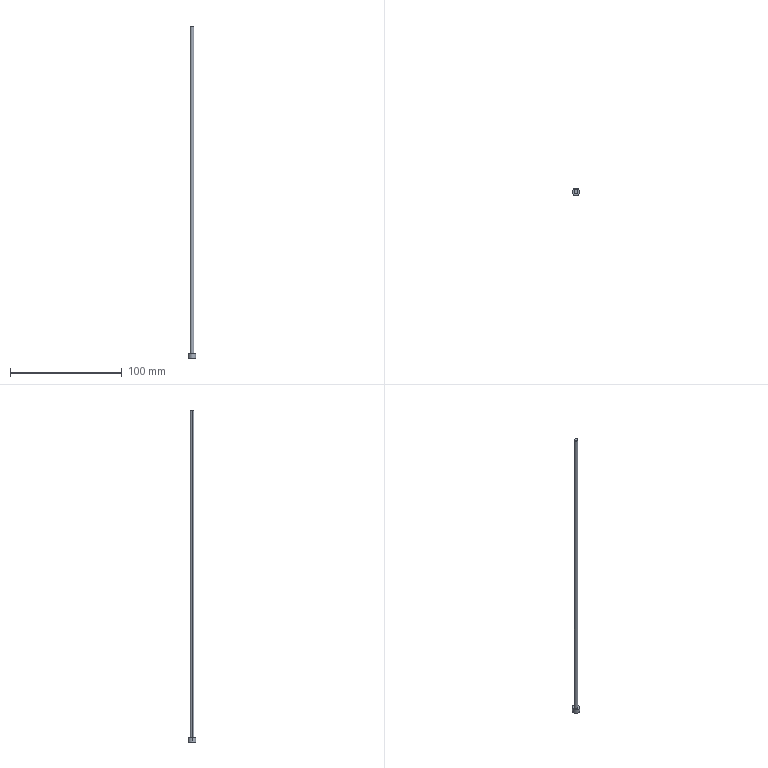Part | Creo | 1 solid | 7 faces | box 7 x 7 x 297.407 mm | volume 2977 mm3 | cylinder 4 | plane 3 | commonest cylinder face diameters 3.5 x2 7 x2
STEP:
#1=CARTESIAN_POINT('',(-36.75,142.5,-292.));
#2=VERTEX_POINT('',#1);
#3=CARTESIAN_POINT('',(-40.25,142.5,-292.));
#4=VERTEX_POINT('',#3);
#5=CARTESIAN_POINT('',(-38.5,142.5,-292.));
#6=DIRECTION('',(0.,0.,-1.));
#7=DIRECTION('',(1.,0.,0.));
#8=AXIS2_PLACEMENT_3D('',#5,#6,#7);
#9=CIRCLE('',#8,1.75);
#10=EDGE_CURVE('',#2,#4,#9,.T.);
#11=ORIENTED_EDGE('',*,*,#10,.T.);
#12=CARTESIAN_POINT('',(-40.25,142.5,1.407));
#13=VERTEX_POINT('',#12);
#14=CARTESIAN_POINT('',(-40.25,142.5,1.407));
#15=DIRECTION('',(0.,0.,-1.));
#16=VECTOR('',#15,293.407);
#17=LINE('',#14,#16);
#18=EDGE_CURVE('',#13,#4,#17,.T.);
#19=ORIENTED_EDGE('',*,*,#18,.F.);
#20=CARTESIAN_POINT('',(-36.75,142.5,1.407));
#21=VERTEX_POINT('',#20);
#22=CARTESIAN_POINT('',(-38.5,142.5,1.407));
#23=DIRECTION('',(0.,0.,1.));
#24=DIRECTION('',(-1.,0.,0.));
#25=AXIS2_PLACEMENT_3D('',#22,#23,#24);
#26=CIRCLE('',#25,1.75);
#27=EDGE_CURVE('',#13,#21,#26,.T.);
#28=ORIENTED_EDGE('',*,*,#27,.T.);
#29=CARTESIAN_POINT('',(-36.75,142.5,1.407));
#30=DIRECTION('',(0.,0.,-1.));
#31=VECTOR('',#30,293.407);
#32=LINE('',#29,#31);
#33=EDGE_CURVE('',#21,#2,#32,.T.);
#34=ORIENTED_EDGE('',*,*,#33,.T.);
#35=EDGE_LOOP('',(#11,#19,#28,#34));
#36=FACE_OUTER_BOUND('',#35,.F.);
#37=CARTESIAN_POINT('',(-38.5,142.5,-5.));
#38=DIRECTION('',(0.,0.,-1.));
#39=DIRECTION('',(1.,0.,0.));
#40=AXIS2_PLACEMENT_3D('',#37,#38,#39);
#41=CYLINDRICAL_SURFACE('',#40,1.75);
#42=ADVANCED_FACE('',(#36),#41,.T.);
#43=CARTESIAN_POINT('',(-35.,142.5,-292.));
#44=VERTEX_POINT('',#43);
#45=CARTESIAN_POINT('',(-42.,142.5,-292.));
#46=VERTEX_POINT('',#45);
#47=CARTESIAN_POINT('',(-38.5,142.5,-292.));
#48=DIRECTION('',(0.,0.,1.));
#49=DIRECTION('',(1.,0.,0.));
#50=AXIS2_PLACEMENT_3D('',#47,#48,#49);
#51=CIRCLE('',#50,3.5);
#52=EDGE_CURVE('',#44,#46,#51,.T.);
#53=ORIENTED_EDGE('',*,*,#52,.F.);
#54=CARTESIAN_POINT('',(-38.5,142.5,-292.));
#55=DIRECTION('',(0.,0.,1.));
#56=DIRECTION('',(-1.,0.,0.));
#57=AXIS2_PLACEMENT_3D('',#54,#55,#56);
#58=CIRCLE('',#57,3.5);
#59=EDGE_CURVE('',#46,#44,#58,.T.);
#60=ORIENTED_EDGE('',*,*,#59,.F.);
#61=EDGE_LOOP('',(#53,#60));
#62=FACE_OUTER_BOUND('',#61,.F.);
#63=ORIENTED_EDGE('',*,*,#10,.F.);
#64=CARTESIAN_POINT('',(-38.5,142.5,-292.));
#65=DIRECTION('',(0.,0.,-1.));
#66=DIRECTION('',(-1.,0.,0.));
#67=AXIS2_PLACEMENT_3D('',#64,#65,#66);
#68=CIRCLE('',#67,1.75);
#69=EDGE_CURVE('',#4,#2,#68,.T.);
#70=ORIENTED_EDGE('',*,*,#69,.F.);
#71=EDGE_LOOP('',(#63,#70));
#72=FACE_BOUND('',#71,.F.);
#73=CARTESIAN_POINT('',(-38.5,142.5,-292.));
#74=DIRECTION('',(0.,0.,1.));
#75=DIRECTION('',(-1.,0.,0.));
#76=AXIS2_PLACEMENT_3D('',#73,#74,#75);
#77=PLANE('',#76);
#78=ADVANCED_FACE('',(#62,#72),#77,.T.);
#79=ORIENTED_EDGE('',*,*,#69,.T.);
#80=ORIENTED_EDGE('',*,*,#33,.F.);
#81=CARTESIAN_POINT('',(-38.5,142.5,1.407));
#82=DIRECTION('',(0.,0.,1.));
#83=DIRECTION('',(1.,0.,0.));
#84=AXIS2_PLACEMENT_3D('',#81,#82,#83);
#85=CIRCLE('',#84,1.75);
#86=EDGE_CURVE('',#21,#13,#85,.T.);
#87=ORIENTED_EDGE('',*,*,#86,.T.);
#88=ORIENTED_EDGE('',*,*,#18,.T.);
#89=EDGE_LOOP('',(#79,#80,#87,#88));
#90=FACE_OUTER_BOUND('',#89,.F.);
#91=CARTESIAN_POINT('',(-38.5,142.5,-5.));
#92=DIRECTION('',(0.,0.,-1.));
#93=DIRECTION('',(1.,0.,0.));
#94=AXIS2_PLACEMENT_3D('',#91,#92,#93);
#95=CYLINDRICAL_SURFACE('',#94,1.75);
#96=ADVANCED_FACE('',(#90),#95,.T.);
#97=ORIENTED_EDGE('',*,*,#86,.F.);
#98=ORIENTED_EDGE('',*,*,#27,.F.);
#99=EDGE_LOOP('',(#97,#98));
#100=FACE_OUTER_BOUND('',#99,.F.);
#101=CARTESIAN_POINT('',(0.,0.,1.407));
#102=DIRECTION('',(0.,0.,1.));
#103=DIRECTION('',(0.,-1.,0.));
#104=AXIS2_PLACEMENT_3D('',#101,#102,#103);
#105=PLANE('',#104);
#106=ADVANCED_FACE('',(#100),#105,.T.);
#107=ORIENTED_EDGE('',*,*,#52,.T.);
#108=CARTESIAN_POINT('',(-42.,142.5,-296.));
#109=VERTEX_POINT('',#108);
#110=CARTESIAN_POINT('',(-42.,142.5,-296.));
#111=DIRECTION('',(0.,0.,1.));
#112=VECTOR('',#111,4.);
#113=LINE('',#110,#112);
#114=EDGE_CURVE('',#109,#46,#113,.T.);
#115=ORIENTED_EDGE('',*,*,#114,.F.);
#116=CARTESIAN_POINT('',(-35.,142.5,-296.));
#117=VERTEX_POINT('',#116);
#118=CARTESIAN_POINT('',(-38.5,142.5,-296.));
#119=DIRECTION('',(0.,0.,-1.));
#120=DIRECTION('',(-1.,0.,0.));
#121=AXIS2_PLACEMENT_3D('',#118,#119,#120);
#122=CIRCLE('',#121,3.5);
#123=EDGE_CURVE('',#109,#117,#122,.T.);
#124=ORIENTED_EDGE('',*,*,#123,.T.);
#125=CARTESIAN_POINT('',(-35.,142.5,-296.));
#126=DIRECTION('',(0.,0.,1.));
#127=VECTOR('',#126,4.);
#128=LINE('',#125,#127);
#129=EDGE_CURVE('',#117,#44,#128,.T.);
#130=ORIENTED_EDGE('',*,*,#129,.T.);
#131=EDGE_LOOP('',(#107,#115,#124,#130));
#132=FACE_OUTER_BOUND('',#131,.F.);
#133=CARTESIAN_POINT('',(-38.5,142.5,-296.));
#134=DIRECTION('',(0.,0.,1.));
#135=DIRECTION('',(-1.,0.,0.));
#136=AXIS2_PLACEMENT_3D('',#133,#134,#135);
#137=CYLINDRICAL_SURFACE('',#136,3.5);
#138=ADVANCED_FACE('',(#132),#137,.T.);
#139=ORIENTED_EDGE('',*,*,#59,.T.);
#140=ORIENTED_EDGE('',*,*,#129,.F.);
#141=CARTESIAN_POINT('',(-38.5,142.5,-296.));
#142=DIRECTION('',(0.,0.,-1.));
#143=DIRECTION('',(1.,0.,0.));
#144=AXIS2_PLACEMENT_3D('',#141,#142,#143);
#145=CIRCLE('',#144,3.5);
#146=EDGE_CURVE('',#117,#109,#145,.T.);
#147=ORIENTED_EDGE('',*,*,#146,.T.);
#148=ORIENTED_EDGE('',*,*,#114,.T.);
#149=EDGE_LOOP('',(#139,#140,#147,#148));
#150=FACE_OUTER_BOUND('',#149,.F.);
#151=CARTESIAN_POINT('',(-38.5,142.5,-296.));
#152=DIRECTION('',(0.,0.,1.));
#153=DIRECTION('',(-1.,0.,0.));
#154=AXIS2_PLACEMENT_3D('',#151,#152,#153);
#155=CYLINDRICAL_SURFACE('',#154,3.5);
#156=ADVANCED_FACE('',(#150),#155,.T.);
#157=ORIENTED_EDGE('',*,*,#146,.F.);
#158=ORIENTED_EDGE('',*,*,#123,.F.);
#159=EDGE_LOOP('',(#157,#158));
#160=FACE_OUTER_BOUND('',#159,.F.);
#161=CARTESIAN_POINT('',(7.7,2.155,-296.));
#162=DIRECTION('',(0.,0.,1.));
#163=DIRECTION('',(0.,-1.,0.));
#164=AXIS2_PLACEMENT_3D('',#161,#162,#163);
#165=PLANE('',#164);
#166=ADVANCED_FACE('',(#160),#165,.F.);
#167=CLOSED_SHELL('',(#42,#78,#96,#106,#138,#156,#166));
#168=MANIFOLD_SOLID_BREP('',#167);
#169=(LENGTH_UNIT()NAMED_UNIT(*)SI_UNIT(.MILLI.,.METRE.));
#170=UNCERTAINTY_MEASURE_WITH_UNIT(LENGTH_MEASURE(0.02976),#169,'','');
#171=(NAMED_UNIT(*)PLANE_ANGLE_UNIT()SI_UNIT($,.RADIAN.));
#172=PLANE_ANGLE_MEASURE_WITH_UNIT(PLANE_ANGLE_MEASURE(0.01745),#171);
#173=(CONVERSION_BASED_UNIT('DEGREE',#172)NAMED_UNIT(*)PLANE_ANGLE_UNIT());
#174=(NAMED_UNIT(*)SI_UNIT($,.STERADIAN.)SOLID_ANGLE_UNIT());
#175=(GEOMETRIC_REPRESENTATION_CONTEXT(3)GLOBAL_UNCERTAINTY_ASSIGNED_CONTEXT((#170))GLOBAL_UNIT_ASSIGNED_CONTEXT((#169,#173,#174))REPRESENTATION_CONTEXT('',''));
#176=ADVANCED_BREP_SHAPE_REPRESENTATION('',(#168),#175);